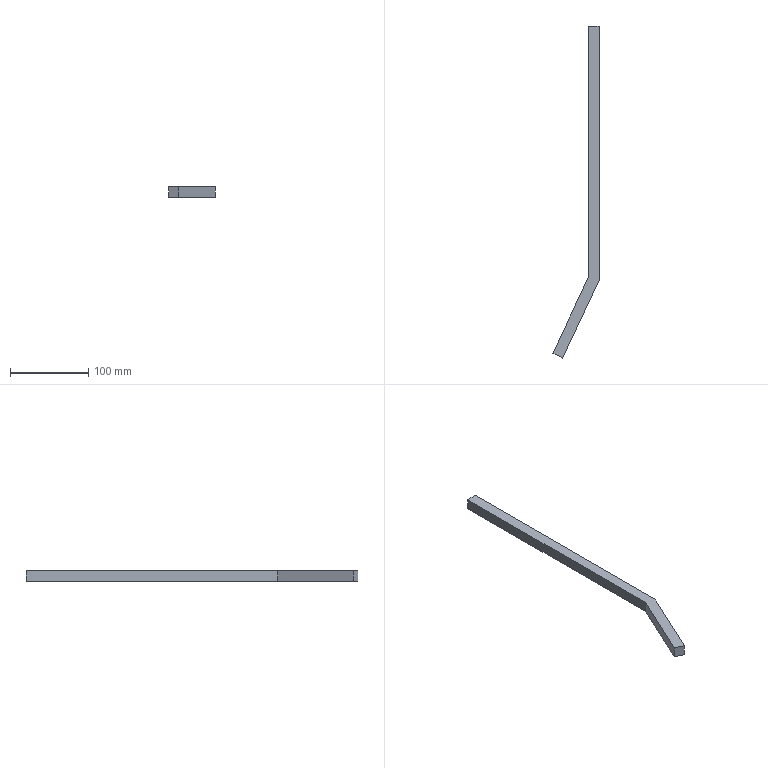Part | NX | features solid 2 | 1 solid | 8 faces | box 59.176 x 424.694 x 14 mm | volume 84652 mm3 | plane 8
STEP:
#1=CARTESIAN_POINT('',(-299.,13.104,-5.));
#2=VERTEX_POINT('',#1);
#3=CARTESIAN_POINT('',(-344.176,-83.777,-5.));
#4=VERTEX_POINT('',#3);
#5=CARTESIAN_POINT('',(-312.48,-15.804,-5.));
#6=DIRECTION('',(-0.4226,-0.9063,0.));
#7=VECTOR('',#6,1000.);
#8=LINE('',#5,#7);
#9=EDGE_CURVE('',#2,#4,#8,.T.);
#10=ORIENTED_EDGE('',*,*,#9,.T.);
#11=CARTESIAN_POINT('',(-344.176,-83.777,9.));
#12=VERTEX_POINT('',#11);
#13=CARTESIAN_POINT('',(-344.176,-83.777,9.));
#14=DIRECTION('',(0.,0.,-1.));
#15=VECTOR('',#14,1000.);
#16=LINE('',#13,#15);
#17=EDGE_CURVE('',#12,#4,#16,.T.);
#18=ORIENTED_EDGE('',*,*,#17,.F.);
#19=CARTESIAN_POINT('',(-299.,13.104,9.));
#20=VERTEX_POINT('',#19);
#21=CARTESIAN_POINT('',(-312.48,-15.804,9.));
#22=DIRECTION('',(-0.4226,-0.9063,0.));
#23=VECTOR('',#22,1000.);
#24=LINE('',#21,#23);
#25=EDGE_CURVE('',#20,#12,#24,.T.);
#26=ORIENTED_EDGE('',*,*,#25,.F.);
#27=CARTESIAN_POINT('',(-299.,13.104,9.));
#28=DIRECTION('',(0.,0.,-1.));
#29=VECTOR('',#28,1000.);
#30=LINE('',#27,#29);
#31=EDGE_CURVE('',#20,#2,#30,.T.);
#32=ORIENTED_EDGE('',*,*,#31,.T.);
#33=EDGE_LOOP('',(#10,#18,#26,#32));
#34=FACE_BOUND('',#33,.T.);
#35=CARTESIAN_POINT('',(-312.48,-15.804,9.));
#36=DIRECTION('',(0.9063,-0.4226,0.));
#37=DIRECTION('',(0.4226,0.9063,0.));
#38=AXIS2_PLACEMENT_3D('',#35,#36,#37);
#39=PLANE('',#38);
#40=ADVANCED_FACE('',(#34),#39,.F.);
#41=CARTESIAN_POINT('',(-331.488,-89.694,-5.));
#42=VERTEX_POINT('',#41);
#43=CARTESIAN_POINT('',(-331.488,-89.694,-5.));
#44=DIRECTION('',(-0.9063,0.4226,0.));
#45=VECTOR('',#44,1000.);
#46=LINE('',#43,#45);
#47=EDGE_CURVE('',#42,#4,#46,.T.);
#48=ORIENTED_EDGE('',*,*,#47,.F.);
#49=CARTESIAN_POINT('',(-331.488,-89.694,9.));
#50=VERTEX_POINT('',#49);
#51=CARTESIAN_POINT('',(-331.488,-89.694,9.));
#52=DIRECTION('',(0.,0.,-1.));
#53=VECTOR('',#52,1000.);
#54=LINE('',#51,#53);
#55=EDGE_CURVE('',#50,#42,#54,.T.);
#56=ORIENTED_EDGE('',*,*,#55,.F.);
#57=CARTESIAN_POINT('',(-331.488,-89.694,9.));
#58=DIRECTION('',(-0.9063,0.4226,0.));
#59=VECTOR('',#58,1000.);
#60=LINE('',#57,#59);
#61=EDGE_CURVE('',#50,#12,#60,.T.);
#62=ORIENTED_EDGE('',*,*,#61,.T.);
#63=ORIENTED_EDGE('',*,*,#17,.T.);
#64=EDGE_LOOP('',(#48,#56,#62,#63));
#65=FACE_BOUND('',#64,.T.);
#66=CARTESIAN_POINT('',(-331.488,-89.694,9.));
#67=DIRECTION('',(-0.4226,-0.9063,0.));
#68=DIRECTION('',(0.9063,-0.4226,0.));
#69=AXIS2_PLACEMENT_3D('',#66,#67,#68);
#70=PLANE('',#69);
#71=ADVANCED_FACE('',(#65),#70,.T.);
#72=CARTESIAN_POINT('',(-285.,10.,-5.));
#73=VERTEX_POINT('',#72);
#74=CARTESIAN_POINT('',(-285.,10.,-5.));
#75=DIRECTION('',(-0.4226,-0.9063,0.));
#76=VECTOR('',#75,1000.);
#77=LINE('',#74,#76);
#78=EDGE_CURVE('',#73,#42,#77,.T.);
#79=ORIENTED_EDGE('',*,*,#78,.F.);
#80=CARTESIAN_POINT('',(-285.,10.,9.));
#81=VERTEX_POINT('',#80);
#82=CARTESIAN_POINT('',(-285.,10.,9.));
#83=DIRECTION('',(0.,0.,-1.));
#84=VECTOR('',#83,1000.);
#85=LINE('',#82,#84);
#86=EDGE_CURVE('',#81,#73,#85,.T.);
#87=ORIENTED_EDGE('',*,*,#86,.F.);
#88=CARTESIAN_POINT('',(-285.,10.,9.));
#89=DIRECTION('',(-0.4226,-0.9063,0.));
#90=VECTOR('',#89,1000.);
#91=LINE('',#88,#90);
#92=EDGE_CURVE('',#81,#50,#91,.T.);
#93=ORIENTED_EDGE('',*,*,#92,.T.);
#94=ORIENTED_EDGE('',*,*,#55,.T.);
#95=EDGE_LOOP('',(#79,#87,#93,#94));
#96=FACE_BOUND('',#95,.T.);
#97=CARTESIAN_POINT('',(-285.,10.,9.));
#98=DIRECTION('',(0.9063,-0.4226,0.));
#99=DIRECTION('',(0.4226,0.9063,0.));
#100=AXIS2_PLACEMENT_3D('',#97,#98,#99);
#101=PLANE('',#100);
#102=ADVANCED_FACE('',(#96),#101,.T.);
#103=CARTESIAN_POINT('',(-285.,335.,-5.));
#104=VERTEX_POINT('',#103);
#105=CARTESIAN_POINT('',(-285.,335.,-5.));
#106=DIRECTION('',(0.,-1.,0.));
#107=VECTOR('',#106,1000.);
#108=LINE('',#105,#107);
#109=EDGE_CURVE('',#104,#73,#108,.T.);
#110=ORIENTED_EDGE('',*,*,#109,.F.);
#111=CARTESIAN_POINT('',(-285.,335.,9.));
#112=VERTEX_POINT('',#111);
#113=CARTESIAN_POINT('',(-285.,335.,9.));
#114=DIRECTION('',(0.,0.,-1.));
#115=VECTOR('',#114,1000.);
#116=LINE('',#113,#115);
#117=EDGE_CURVE('',#112,#104,#116,.T.);
#118=ORIENTED_EDGE('',*,*,#117,.F.);
#119=CARTESIAN_POINT('',(-285.,335.,9.));
#120=DIRECTION('',(0.,-1.,0.));
#121=VECTOR('',#120,1000.);
#122=LINE('',#119,#121);
#123=EDGE_CURVE('',#112,#81,#122,.T.);
#124=ORIENTED_EDGE('',*,*,#123,.T.);
#125=ORIENTED_EDGE('',*,*,#86,.T.);
#126=EDGE_LOOP('',(#110,#118,#124,#125));
#127=FACE_BOUND('',#126,.T.);
#128=CARTESIAN_POINT('',(-285.,335.,9.));
#129=DIRECTION('',(1.,0.,0.));
#130=DIRECTION('',(0.,0.,-1.));
#131=AXIS2_PLACEMENT_3D('',#128,#129,#130);
#132=PLANE('',#131);
#133=ADVANCED_FACE('',(#127),#132,.T.);
#134=CARTESIAN_POINT('',(-299.,335.,-5.));
#135=VERTEX_POINT('',#134);
#136=CARTESIAN_POINT('',(-285.,335.,-5.));
#137=DIRECTION('',(-1.,0.,0.));
#138=VECTOR('',#137,1000.);
#139=LINE('',#136,#138);
#140=EDGE_CURVE('',#104,#135,#139,.T.);
#141=ORIENTED_EDGE('',*,*,#140,.T.);
#142=CARTESIAN_POINT('',(-299.,335.,9.));
#143=VERTEX_POINT('',#142);
#144=CARTESIAN_POINT('',(-299.,335.,9.));
#145=DIRECTION('',(0.,0.,-1.));
#146=VECTOR('',#145,1000.);
#147=LINE('',#144,#146);
#148=EDGE_CURVE('',#143,#135,#147,.T.);
#149=ORIENTED_EDGE('',*,*,#148,.F.);
#150=CARTESIAN_POINT('',(-285.,335.,9.));
#151=DIRECTION('',(-1.,0.,0.));
#152=VECTOR('',#151,1000.);
#153=LINE('',#150,#152);
#154=EDGE_CURVE('',#112,#143,#153,.T.);
#155=ORIENTED_EDGE('',*,*,#154,.F.);
#156=ORIENTED_EDGE('',*,*,#117,.T.);
#157=EDGE_LOOP('',(#141,#149,#155,#156));
#158=FACE_BOUND('',#157,.T.);
#159=CARTESIAN_POINT('',(-285.,335.,9.));
#160=DIRECTION('',(0.,-1.,0.));
#161=DIRECTION('',(0.,0.,-1.));
#162=AXIS2_PLACEMENT_3D('',#159,#160,#161);
#163=PLANE('',#162);
#164=ADVANCED_FACE('',(#158),#163,.F.);
#165=CARTESIAN_POINT('',(-299.,335.,-5.));
#166=DIRECTION('',(0.,-1.,0.));
#167=VECTOR('',#166,1000.);
#168=LINE('',#165,#167);
#169=EDGE_CURVE('',#135,#2,#168,.T.);
#170=ORIENTED_EDGE('',*,*,#169,.T.);
#171=ORIENTED_EDGE('',*,*,#31,.F.);
#172=CARTESIAN_POINT('',(-299.,335.,9.));
#173=DIRECTION('',(0.,-1.,0.));
#174=VECTOR('',#173,1000.);
#175=LINE('',#172,#174);
#176=EDGE_CURVE('',#143,#20,#175,.T.);
#177=ORIENTED_EDGE('',*,*,#176,.F.);
#178=ORIENTED_EDGE('',*,*,#148,.T.);
#179=EDGE_LOOP('',(#170,#171,#177,#178));
#180=FACE_BOUND('',#179,.T.);
#181=CARTESIAN_POINT('',(-299.,335.,9.));
#182=DIRECTION('',(1.,0.,0.));
#183=DIRECTION('',(0.,0.,-1.));
#184=AXIS2_PLACEMENT_3D('',#181,#182,#183);
#185=PLANE('',#184);
#186=ADVANCED_FACE('',(#180),#185,.F.);
#187=ORIENTED_EDGE('',*,*,#176,.T.);
#188=ORIENTED_EDGE('',*,*,#25,.T.);
#189=ORIENTED_EDGE('',*,*,#61,.F.);
#190=ORIENTED_EDGE('',*,*,#92,.F.);
#191=ORIENTED_EDGE('',*,*,#123,.F.);
#192=ORIENTED_EDGE('',*,*,#154,.T.);
#193=EDGE_LOOP('',(#187,#188,#189,#190,#191,#192));
#194=FACE_BOUND('',#193,.T.);
#195=CARTESIAN_POINT('',(-299.,335.,9.));
#196=DIRECTION('',(0.,0.,-1.));
#197=DIRECTION('',(-1.,0.,0.));
#198=AXIS2_PLACEMENT_3D('',#195,#196,#197);
#199=PLANE('',#198);
#200=ADVANCED_FACE('',(#194),#199,.F.);
#201=ORIENTED_EDGE('',*,*,#9,.F.);
#202=ORIENTED_EDGE('',*,*,#169,.F.);
#203=ORIENTED_EDGE('',*,*,#140,.F.);
#204=ORIENTED_EDGE('',*,*,#109,.T.);
#205=ORIENTED_EDGE('',*,*,#78,.T.);
#206=ORIENTED_EDGE('',*,*,#47,.T.);
#207=EDGE_LOOP('',(#201,#202,#203,#204,#205,#206));
#208=FACE_BOUND('',#207,.T.);
#209=CARTESIAN_POINT('',(-299.,335.,-5.));
#210=DIRECTION('',(0.,0.,-1.));
#211=DIRECTION('',(-1.,0.,0.));
#212=AXIS2_PLACEMENT_3D('',#209,#210,#211);
#213=PLANE('',#212);
#214=ADVANCED_FACE('',(#208),#213,.T.);
#215=CLOSED_SHELL('',(#40,#71,#102,#133,#164,#186,#200,#214));
#216=MANIFOLD_SOLID_BREP('',#215);
#217=(LENGTH_UNIT()NAMED_UNIT(*)SI_UNIT(.MILLI.,.METRE.));
#218=UNCERTAINTY_MEASURE_WITH_UNIT(LENGTH_MEASURE(0.00001),#217,'','');
#219=(NAMED_UNIT(*)PLANE_ANGLE_UNIT()SI_UNIT($,.RADIAN.));
#220=(NAMED_UNIT(*)SI_UNIT($,.STERADIAN.)SOLID_ANGLE_UNIT());
#221=(GEOMETRIC_REPRESENTATION_CONTEXT(3)GLOBAL_UNCERTAINTY_ASSIGNED_CONTEXT((#218))GLOBAL_UNIT_ASSIGNED_CONTEXT((#217,#219,#220))REPRESENTATION_CONTEXT('',''));
#222=ADVANCED_BREP_SHAPE_REPRESENTATION('',(#216),#221);